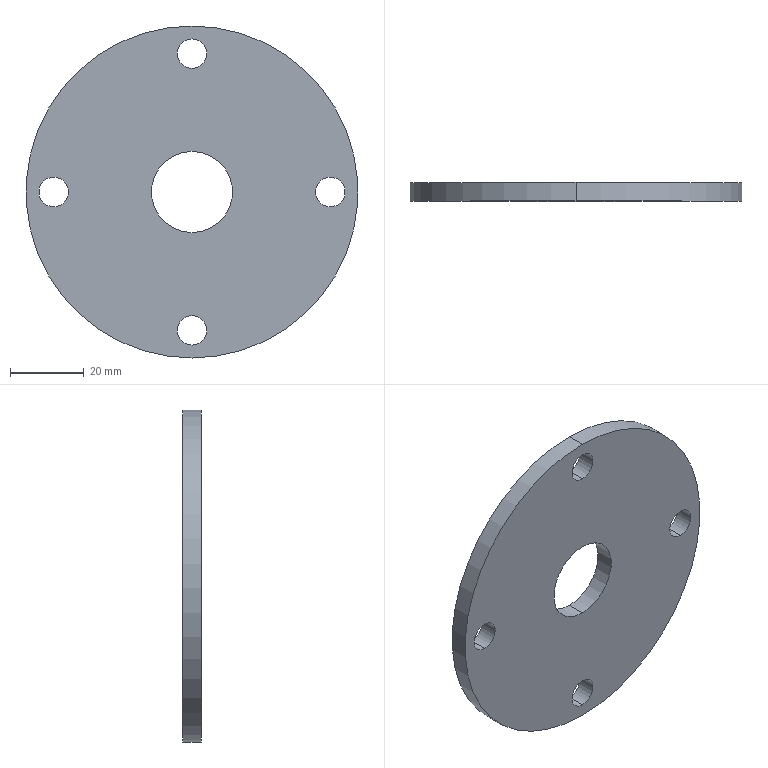Part | STEP file | Guide wheel mechanism revised.sldasm-Part-427 | 1 solid | 34 faces | box 90 x 5 x 90 mm | volume 28260 mm3 | plane 22 | cylinder 12 | commonest cylinder face diameters 8 x8 22 x2 90 x2
STEP:
#1=CARTESIAN_POINT('',(37.5,5.,-4.));
#2=VERTEX_POINT('',#1);
#3=CARTESIAN_POINT('',(37.5,5.,4.));
#4=VERTEX_POINT('',#3);
#5=CARTESIAN_POINT('',(37.5,5.,0.));
#6=DIRECTION('',(0.,1.,0.));
#7=DIRECTION('',(0.,0.,1.));
#8=AXIS2_PLACEMENT_3D('',#5,#6,#7);
#9=CIRCLE('',#8,4.);
#10=EDGE_CURVE('',#2,#4,#9,.T.);
#11=ORIENTED_EDGE('',*,*,#10,.T.);
#12=CARTESIAN_POINT('',(37.5,0.,4.));
#13=VERTEX_POINT('',#12);
#14=CARTESIAN_POINT('',(37.5,5.,4.));
#15=DIRECTION('',(0.,-1.,0.));
#16=VECTOR('',#15,1000.);
#17=LINE('',#14,#16);
#18=EDGE_CURVE('',#4,#13,#17,.T.);
#19=ORIENTED_EDGE('',*,*,#18,.T.);
#20=CARTESIAN_POINT('',(37.5,0.,-4.));
#21=VERTEX_POINT('',#20);
#22=CARTESIAN_POINT('',(37.5,0.,0.));
#23=DIRECTION('',(0.,1.,0.));
#24=DIRECTION('',(0.,0.,1.));
#25=AXIS2_PLACEMENT_3D('',#22,#23,#24);
#26=CIRCLE('',#25,4.);
#27=EDGE_CURVE('',#21,#13,#26,.T.);
#28=ORIENTED_EDGE('',*,*,#27,.F.);
#29=CARTESIAN_POINT('',(37.5,5.,-4.));
#30=DIRECTION('',(0.,-1.,0.));
#31=VECTOR('',#30,1000.);
#32=LINE('',#29,#31);
#33=EDGE_CURVE('',#2,#21,#32,.T.);
#34=ORIENTED_EDGE('',*,*,#33,.F.);
#35=EDGE_LOOP('',(#11,#19,#28,#34));
#36=FACE_OUTER_BOUND('',#35,.T.);
#37=CARTESIAN_POINT('',(37.5,5.,0.));
#38=DIRECTION('',(0.,-1.,0.));
#39=DIRECTION('',(0.,0.,-1.));
#40=AXIS2_PLACEMENT_3D('',#37,#38,#39);
#41=CYLINDRICAL_SURFACE('',#40,4.);
#42=ADVANCED_FACE('',(#36),#41,.F.);
#43=CARTESIAN_POINT('',(0.,5.,33.5));
#44=VERTEX_POINT('',#43);
#45=CARTESIAN_POINT('',(0.,5.,41.5));
#46=VERTEX_POINT('',#45);
#47=CARTESIAN_POINT('',(0.,5.,37.5));
#48=DIRECTION('',(0.,1.,0.));
#49=DIRECTION('',(0.,0.,1.));
#50=AXIS2_PLACEMENT_3D('',#47,#48,#49);
#51=CIRCLE('',#50,4.);
#52=EDGE_CURVE('',#44,#46,#51,.T.);
#53=ORIENTED_EDGE('',*,*,#52,.T.);
#54=CARTESIAN_POINT('',(0.,0.,41.5));
#55=VERTEX_POINT('',#54);
#56=CARTESIAN_POINT('',(0.,5.,41.5));
#57=DIRECTION('',(0.,-1.,0.));
#58=VECTOR('',#57,1000.);
#59=LINE('',#56,#58);
#60=EDGE_CURVE('',#46,#55,#59,.T.);
#61=ORIENTED_EDGE('',*,*,#60,.T.);
#62=CARTESIAN_POINT('',(0.,0.,33.5));
#63=VERTEX_POINT('',#62);
#64=CARTESIAN_POINT('',(0.,0.,37.5));
#65=DIRECTION('',(0.,1.,0.));
#66=DIRECTION('',(0.,0.,1.));
#67=AXIS2_PLACEMENT_3D('',#64,#65,#66);
#68=CIRCLE('',#67,4.);
#69=EDGE_CURVE('',#63,#55,#68,.T.);
#70=ORIENTED_EDGE('',*,*,#69,.F.);
#71=CARTESIAN_POINT('',(0.,5.,33.5));
#72=DIRECTION('',(0.,-1.,0.));
#73=VECTOR('',#72,1000.);
#74=LINE('',#71,#73);
#75=EDGE_CURVE('',#44,#63,#74,.T.);
#76=ORIENTED_EDGE('',*,*,#75,.F.);
#77=EDGE_LOOP('',(#53,#61,#70,#76));
#78=FACE_OUTER_BOUND('',#77,.T.);
#79=CARTESIAN_POINT('',(0.,5.,37.5));
#80=DIRECTION('',(0.,-1.,0.));
#81=DIRECTION('',(0.,0.,-1.));
#82=AXIS2_PLACEMENT_3D('',#79,#80,#81);
#83=CYLINDRICAL_SURFACE('',#82,4.);
#84=ADVANCED_FACE('',(#78),#83,.F.);
#85=CARTESIAN_POINT('',(-37.5,5.,-4.));
#86=VERTEX_POINT('',#85);
#87=CARTESIAN_POINT('',(-37.5,5.,4.));
#88=VERTEX_POINT('',#87);
#89=CARTESIAN_POINT('',(-37.5,5.,0.));
#90=DIRECTION('',(0.,1.,0.));
#91=DIRECTION('',(0.,0.,1.));
#92=AXIS2_PLACEMENT_3D('',#89,#90,#91);
#93=CIRCLE('',#92,4.);
#94=EDGE_CURVE('',#86,#88,#93,.T.);
#95=ORIENTED_EDGE('',*,*,#94,.T.);
#96=CARTESIAN_POINT('',(-37.5,0.,4.));
#97=VERTEX_POINT('',#96);
#98=CARTESIAN_POINT('',(-37.5,5.,4.));
#99=DIRECTION('',(0.,-1.,0.));
#100=VECTOR('',#99,1000.);
#101=LINE('',#98,#100);
#102=EDGE_CURVE('',#88,#97,#101,.T.);
#103=ORIENTED_EDGE('',*,*,#102,.T.);
#104=CARTESIAN_POINT('',(-37.5,0.,-4.));
#105=VERTEX_POINT('',#104);
#106=CARTESIAN_POINT('',(-37.5,0.,0.));
#107=DIRECTION('',(0.,1.,0.));
#108=DIRECTION('',(0.,0.,1.));
#109=AXIS2_PLACEMENT_3D('',#106,#107,#108);
#110=CIRCLE('',#109,4.);
#111=EDGE_CURVE('',#105,#97,#110,.T.);
#112=ORIENTED_EDGE('',*,*,#111,.F.);
#113=CARTESIAN_POINT('',(-37.5,5.,-4.));
#114=DIRECTION('',(0.,-1.,0.));
#115=VECTOR('',#114,1000.);
#116=LINE('',#113,#115);
#117=EDGE_CURVE('',#86,#105,#116,.T.);
#118=ORIENTED_EDGE('',*,*,#117,.F.);
#119=EDGE_LOOP('',(#95,#103,#112,#118));
#120=FACE_OUTER_BOUND('',#119,.T.);
#121=CARTESIAN_POINT('',(-37.5,5.,0.));
#122=DIRECTION('',(0.,-1.,0.));
#123=DIRECTION('',(0.,0.,-1.));
#124=AXIS2_PLACEMENT_3D('',#121,#122,#123);
#125=CYLINDRICAL_SURFACE('',#124,4.);
#126=ADVANCED_FACE('',(#120),#125,.F.);
#127=CARTESIAN_POINT('',(0.,5.,-41.5));
#128=VERTEX_POINT('',#127);
#129=CARTESIAN_POINT('',(0.,5.,-33.5));
#130=VERTEX_POINT('',#129);
#131=CARTESIAN_POINT('',(0.,5.,-37.5));
#132=DIRECTION('',(0.,1.,0.));
#133=DIRECTION('',(0.,0.,1.));
#134=AXIS2_PLACEMENT_3D('',#131,#132,#133);
#135=CIRCLE('',#134,4.);
#136=EDGE_CURVE('',#128,#130,#135,.T.);
#137=ORIENTED_EDGE('',*,*,#136,.T.);
#138=CARTESIAN_POINT('',(0.,0.,-33.5));
#139=VERTEX_POINT('',#138);
#140=CARTESIAN_POINT('',(0.,5.,-33.5));
#141=DIRECTION('',(0.,-1.,0.));
#142=VECTOR('',#141,1000.);
#143=LINE('',#140,#142);
#144=EDGE_CURVE('',#130,#139,#143,.T.);
#145=ORIENTED_EDGE('',*,*,#144,.T.);
#146=CARTESIAN_POINT('',(0.,0.,-41.5));
#147=VERTEX_POINT('',#146);
#148=CARTESIAN_POINT('',(0.,0.,-37.5));
#149=DIRECTION('',(0.,1.,0.));
#150=DIRECTION('',(0.,0.,1.));
#151=AXIS2_PLACEMENT_3D('',#148,#149,#150);
#152=CIRCLE('',#151,4.);
#153=EDGE_CURVE('',#147,#139,#152,.T.);
#154=ORIENTED_EDGE('',*,*,#153,.F.);
#155=CARTESIAN_POINT('',(0.,5.,-41.5));
#156=DIRECTION('',(0.,-1.,0.));
#157=VECTOR('',#156,1000.);
#158=LINE('',#155,#157);
#159=EDGE_CURVE('',#128,#147,#158,.T.);
#160=ORIENTED_EDGE('',*,*,#159,.F.);
#161=EDGE_LOOP('',(#137,#145,#154,#160));
#162=FACE_OUTER_BOUND('',#161,.T.);
#163=CARTESIAN_POINT('',(0.,5.,-37.5));
#164=DIRECTION('',(0.,-1.,0.));
#165=DIRECTION('',(0.,0.,-1.));
#166=AXIS2_PLACEMENT_3D('',#163,#164,#165);
#167=CYLINDRICAL_SURFACE('',#166,4.);
#168=ADVANCED_FACE('',(#162),#167,.F.);
#169=CARTESIAN_POINT('',(0.,5.,-11.));
#170=VERTEX_POINT('',#169);
#171=CARTESIAN_POINT('',(0.,5.,11.));
#172=VERTEX_POINT('',#171);
#173=CARTESIAN_POINT('',(0.,5.,0.));
#174=DIRECTION('',(0.,1.,0.));
#175=DIRECTION('',(0.,0.,1.));
#176=AXIS2_PLACEMENT_3D('',#173,#174,#175);
#177=CIRCLE('',#176,11.);
#178=EDGE_CURVE('',#170,#172,#177,.T.);
#179=ORIENTED_EDGE('',*,*,#178,.T.);
#180=CARTESIAN_POINT('',(0.,0.,11.));
#181=VERTEX_POINT('',#180);
#182=CARTESIAN_POINT('',(0.,5.,11.));
#183=DIRECTION('',(0.,-1.,0.));
#184=VECTOR('',#183,1000.);
#185=LINE('',#182,#184);
#186=EDGE_CURVE('',#172,#181,#185,.T.);
#187=ORIENTED_EDGE('',*,*,#186,.T.);
#188=CARTESIAN_POINT('',(0.,0.,-11.));
#189=VERTEX_POINT('',#188);
#190=CARTESIAN_POINT('',(0.,0.,0.));
#191=DIRECTION('',(0.,1.,0.));
#192=DIRECTION('',(0.,0.,1.));
#193=AXIS2_PLACEMENT_3D('',#190,#191,#192);
#194=CIRCLE('',#193,11.);
#195=EDGE_CURVE('',#189,#181,#194,.T.);
#196=ORIENTED_EDGE('',*,*,#195,.F.);
#197=CARTESIAN_POINT('',(0.,5.,-11.));
#198=DIRECTION('',(0.,-1.,0.));
#199=VECTOR('',#198,1000.);
#200=LINE('',#197,#199);
#201=EDGE_CURVE('',#170,#189,#200,.T.);
#202=ORIENTED_EDGE('',*,*,#201,.F.);
#203=EDGE_LOOP('',(#179,#187,#196,#202));
#204=FACE_OUTER_BOUND('',#203,.T.);
#205=CARTESIAN_POINT('',(0.,5.,0.));
#206=DIRECTION('',(0.,-1.,0.));
#207=DIRECTION('',(0.,0.,-1.));
#208=AXIS2_PLACEMENT_3D('',#205,#206,#207);
#209=CYLINDRICAL_SURFACE('',#208,11.);
#210=ADVANCED_FACE('',(#204),#209,.F.);
#211=CARTESIAN_POINT('',(0.,5.,45.));
#212=VERTEX_POINT('',#211);
#213=CARTESIAN_POINT('',(0.,5.,-45.));
#214=VERTEX_POINT('',#213);
#215=CARTESIAN_POINT('',(0.,5.,0.));
#216=DIRECTION('',(0.,1.,0.));
#217=DIRECTION('',(0.,0.,1.));
#218=AXIS2_PLACEMENT_3D('',#215,#216,#217);
#219=CIRCLE('',#218,45.);
#220=EDGE_CURVE('',#212,#214,#219,.T.);
#221=ORIENTED_EDGE('',*,*,#220,.F.);
#222=CARTESIAN_POINT('',(0.,0.,45.));
#223=VERTEX_POINT('',#222);
#224=CARTESIAN_POINT('',(0.,5.,45.));
#225=DIRECTION('',(0.,-1.,0.));
#226=VECTOR('',#225,1000.);
#227=LINE('',#224,#226);
#228=EDGE_CURVE('',#212,#223,#227,.T.);
#229=ORIENTED_EDGE('',*,*,#228,.T.);
#230=CARTESIAN_POINT('',(0.,0.,-45.));
#231=VERTEX_POINT('',#230);
#232=CARTESIAN_POINT('',(0.,0.,0.));
#233=DIRECTION('',(0.,1.,0.));
#234=DIRECTION('',(0.,0.,1.));
#235=AXIS2_PLACEMENT_3D('',#232,#233,#234);
#236=CIRCLE('',#235,45.);
#237=EDGE_CURVE('',#223,#231,#236,.T.);
#238=ORIENTED_EDGE('',*,*,#237,.T.);
#239=CARTESIAN_POINT('',(0.,5.,-45.));
#240=DIRECTION('',(0.,-1.,0.));
#241=VECTOR('',#240,1000.);
#242=LINE('',#239,#241);
#243=EDGE_CURVE('',#214,#231,#242,.T.);
#244=ORIENTED_EDGE('',*,*,#243,.F.);
#245=EDGE_LOOP('',(#221,#229,#238,#244));
#246=FACE_OUTER_BOUND('',#245,.T.);
#247=CARTESIAN_POINT('',(0.,5.,0.));
#248=DIRECTION('',(0.,-1.,0.));
#249=DIRECTION('',(0.,0.,-1.));
#250=AXIS2_PLACEMENT_3D('',#247,#248,#249);
#251=CYLINDRICAL_SURFACE('',#250,45.);
#252=ADVANCED_FACE('',(#246),#251,.T.);
#253=CARTESIAN_POINT('',(-22.309,5.,26.198));
#254=VERTEX_POINT('',#253);
#255=CARTESIAN_POINT('',(-17.147,5.,21.036));
#256=VERTEX_POINT('',#255);
#257=CARTESIAN_POINT('',(1.945,5.,1.945));
#258=DIRECTION('',(0.7071,0.,-0.7071));
#259=VECTOR('',#258,1000.);
#260=LINE('',#257,#259);
#261=EDGE_CURVE('',#254,#256,#260,.T.);
#262=ORIENTED_EDGE('',*,*,#261,.F.);
#263=CARTESIAN_POINT('',(-26.198,5.,22.309));
#264=VERTEX_POINT('',#263);
#265=CARTESIAN_POINT('',(-24.254,5.,24.254));
#266=DIRECTION('',(0.7071,0.,0.7071));
#267=VECTOR('',#266,1000.);
#268=LINE('',#265,#267);
#269=EDGE_CURVE('',#264,#254,#268,.T.);
#270=ORIENTED_EDGE('',*,*,#269,.F.);
#271=CARTESIAN_POINT('',(-21.036,5.,17.147));
#272=VERTEX_POINT('',#271);
#273=CARTESIAN_POINT('',(-1.945,5.,-1.945));
#274=DIRECTION('',(0.7071,0.,-0.7071));
#275=VECTOR('',#274,1000.);
#276=LINE('',#273,#275);
#277=EDGE_CURVE('',#264,#272,#276,.T.);
#278=ORIENTED_EDGE('',*,*,#277,.T.);
#279=CARTESIAN_POINT('',(-19.092,5.,19.092));
#280=DIRECTION('',(0.7071,0.,0.7071));
#281=VECTOR('',#280,1000.);
#282=LINE('',#279,#281);
#283=EDGE_CURVE('',#272,#256,#282,.T.);
#284=ORIENTED_EDGE('',*,*,#283,.T.);
#285=EDGE_LOOP('',(#262,#270,#278,#284));
#286=FACE_BOUND('',#285,.T.);
#287=CARTESIAN_POINT('',(26.198,5.,22.309));
#288=VERTEX_POINT('',#287);
#289=CARTESIAN_POINT('',(21.036,5.,17.147));
#290=VERTEX_POINT('',#289);
#291=CARTESIAN_POINT('',(1.945,5.,-1.945));
#292=DIRECTION('',(-0.7071,0.,-0.7071));
#293=VECTOR('',#292,1000.);
#294=LINE('',#291,#293);
#295=EDGE_CURVE('',#288,#290,#294,.T.);
#296=ORIENTED_EDGE('',*,*,#295,.F.);
#297=CARTESIAN_POINT('',(22.309,5.,26.198));
#298=VERTEX_POINT('',#297);
#299=CARTESIAN_POINT('',(24.254,5.,24.254));
#300=DIRECTION('',(0.7071,0.,-0.7071));
#301=VECTOR('',#300,1000.);
#302=LINE('',#299,#301);
#303=EDGE_CURVE('',#298,#288,#302,.T.);
#304=ORIENTED_EDGE('',*,*,#303,.F.);
#305=CARTESIAN_POINT('',(17.147,5.,21.036));
#306=VERTEX_POINT('',#305);
#307=CARTESIAN_POINT('',(-1.945,5.,1.945));
#308=DIRECTION('',(-0.7071,0.,-0.7071));
#309=VECTOR('',#308,1000.);
#310=LINE('',#307,#309);
#311=EDGE_CURVE('',#298,#306,#310,.T.);
#312=ORIENTED_EDGE('',*,*,#311,.T.);
#313=CARTESIAN_POINT('',(19.092,5.,19.092));
#314=DIRECTION('',(0.7071,0.,-0.7071));
#315=VECTOR('',#314,1000.);
#316=LINE('',#313,#315);
#317=EDGE_CURVE('',#306,#290,#316,.T.);
#318=ORIENTED_EDGE('',*,*,#317,.T.);
#319=EDGE_LOOP('',(#296,#304,#312,#318));
#320=FACE_BOUND('',#319,.T.);
#321=CARTESIAN_POINT('',(22.309,5.,-26.198));
#322=VERTEX_POINT('',#321);
#323=CARTESIAN_POINT('',(17.147,5.,-21.036));
#324=VERTEX_POINT('',#323);
#325=CARTESIAN_POINT('',(-1.945,5.,-1.945));
#326=DIRECTION('',(-0.7071,0.,0.7071));
#327=VECTOR('',#326,1000.);
#328=LINE('',#325,#327);
#329=EDGE_CURVE('',#322,#324,#328,.T.);
#330=ORIENTED_EDGE('',*,*,#329,.F.);
#331=CARTESIAN_POINT('',(26.198,5.,-22.309));
#332=VERTEX_POINT('',#331);
#333=CARTESIAN_POINT('',(24.254,5.,-24.254));
#334=DIRECTION('',(-0.7071,0.,-0.7071));
#335=VECTOR('',#334,1000.);
#336=LINE('',#333,#335);
#337=EDGE_CURVE('',#332,#322,#336,.T.);
#338=ORIENTED_EDGE('',*,*,#337,.F.);
#339=CARTESIAN_POINT('',(21.036,5.,-17.147));
#340=VERTEX_POINT('',#339);
#341=CARTESIAN_POINT('',(1.945,5.,1.945));
#342=DIRECTION('',(-0.7071,0.,0.7071));
#343=VECTOR('',#342,1000.);
#344=LINE('',#341,#343);
#345=EDGE_CURVE('',#332,#340,#344,.T.);
#346=ORIENTED_EDGE('',*,*,#345,.T.);
#347=CARTESIAN_POINT('',(19.092,5.,-19.092));
#348=DIRECTION('',(-0.7071,0.,-0.7071));
#349=VECTOR('',#348,1000.);
#350=LINE('',#347,#349);
#351=EDGE_CURVE('',#340,#324,#350,.T.);
#352=ORIENTED_EDGE('',*,*,#351,.T.);
#353=EDGE_LOOP('',(#330,#338,#346,#352));
#354=FACE_BOUND('',#353,.T.);
#355=CARTESIAN_POINT('',(-26.198,5.,-22.309));
#356=VERTEX_POINT('',#355);
#357=CARTESIAN_POINT('',(-21.036,5.,-17.147));
#358=VERTEX_POINT('',#357);
#359=CARTESIAN_POINT('',(-1.945,5.,1.945));
#360=DIRECTION('',(0.7071,0.,0.7071));
#361=VECTOR('',#360,1000.);
#362=LINE('',#359,#361);
#363=EDGE_CURVE('',#356,#358,#362,.T.);
#364=ORIENTED_EDGE('',*,*,#363,.F.);
#365=CARTESIAN_POINT('',(-22.309,5.,-26.198));
#366=VERTEX_POINT('',#365);
#367=CARTESIAN_POINT('',(-24.254,5.,-24.254));
#368=DIRECTION('',(-0.7071,0.,0.7071));
#369=VECTOR('',#368,1000.);
#370=LINE('',#367,#369);
#371=EDGE_CURVE('',#366,#356,#370,.T.);
#372=ORIENTED_EDGE('',*,*,#371,.F.);
#373=CARTESIAN_POINT('',(-17.147,5.,-21.036));
#374=VERTEX_POINT('',#373);
#375=CARTESIAN_POINT('',(1.945,5.,-1.945));
#376=DIRECTION('',(0.7071,0.,0.7071));
#377=VECTOR('',#376,1000.);
#378=LINE('',#375,#377);
#379=EDGE_CURVE('',#366,#374,#378,.T.);
#380=ORIENTED_EDGE('',*,*,#379,.T.);
#381=CARTESIAN_POINT('',(-19.092,5.,-19.092));
#382=DIRECTION('',(-0.7071,0.,0.7071));
#383=VECTOR('',#382,1000.);
#384=LINE('',#381,#383);
#385=EDGE_CURVE('',#374,#358,#384,.T.);
#386=ORIENTED_EDGE('',*,*,#385,.T.);
#387=EDGE_LOOP('',(#364,#372,#380,#386));
#388=FACE_BOUND('',#387,.T.);
#389=ORIENTED_EDGE('',*,*,#52,.F.);
#390=CARTESIAN_POINT('',(0.,5.,37.5));
#391=DIRECTION('',(0.,1.,0.));
#392=DIRECTION('',(0.,0.,1.));
#393=AXIS2_PLACEMENT_3D('',#390,#391,#392);
#394=CIRCLE('',#393,4.);
#395=EDGE_CURVE('',#46,#44,#394,.T.);
#396=ORIENTED_EDGE('',*,*,#395,.F.);
#397=EDGE_LOOP('',(#389,#396));
#398=FACE_BOUND('',#397,.T.);
#399=ORIENTED_EDGE('',*,*,#136,.F.);
#400=CARTESIAN_POINT('',(0.,5.,-37.5));
#401=DIRECTION('',(0.,1.,0.));
#402=DIRECTION('',(0.,0.,1.));
#403=AXIS2_PLACEMENT_3D('',#400,#401,#402);
#404=CIRCLE('',#403,4.);
#405=EDGE_CURVE('',#130,#128,#404,.T.);
#406=ORIENTED_EDGE('',*,*,#405,.F.);
#407=EDGE_LOOP('',(#399,#406));
#408=FACE_BOUND('',#407,.T.);
#409=CARTESIAN_POINT('',(0.,5.,0.));
#410=DIRECTION('',(0.,1.,0.));
#411=DIRECTION('',(0.,0.,1.));
#412=AXIS2_PLACEMENT_3D('',#409,#410,#411);
#413=CIRCLE('',#412,45.);
#414=EDGE_CURVE('',#214,#212,#413,.T.);
#415=ORIENTED_EDGE('',*,*,#414,.T.);
#416=ORIENTED_EDGE('',*,*,#220,.T.);
#417=EDGE_LOOP('',(#415,#416));
#418=FACE_OUTER_BOUND('',#417,.T.);
#419=ORIENTED_EDGE('',*,*,#178,.F.);
#420=CARTESIAN_POINT('',(0.,5.,0.));
#421=DIRECTION('',(0.,1.,0.));
#422=DIRECTION('',(0.,0.,1.));
#423=AXIS2_PLACEMENT_3D('',#420,#421,#422);
#424=CIRCLE('',#423,11.);
#425=EDGE_CURVE('',#172,#170,#424,.T.);
#426=ORIENTED_EDGE('',*,*,#425,.F.);
#427=EDGE_LOOP('',(#419,#426));
#428=FACE_BOUND('',#427,.T.);
#429=ORIENTED_EDGE('',*,*,#94,.F.);
#430=CARTESIAN_POINT('',(-37.5,5.,0.));
#431=DIRECTION('',(0.,1.,0.));
#432=DIRECTION('',(0.,0.,1.));
#433=AXIS2_PLACEMENT_3D('',#430,#431,#432);
#434=CIRCLE('',#433,4.);
#435=EDGE_CURVE('',#88,#86,#434,.T.);
#436=ORIENTED_EDGE('',*,*,#435,.F.);
#437=EDGE_LOOP('',(#429,#436));
#438=FACE_BOUND('',#437,.T.);
#439=ORIENTED_EDGE('',*,*,#10,.F.);
#440=CARTESIAN_POINT('',(37.5,5.,0.));
#441=DIRECTION('',(0.,1.,0.));
#442=DIRECTION('',(0.,0.,1.));
#443=AXIS2_PLACEMENT_3D('',#440,#441,#442);
#444=CIRCLE('',#443,4.);
#445=EDGE_CURVE('',#4,#2,#444,.T.);
#446=ORIENTED_EDGE('',*,*,#445,.F.);
#447=EDGE_LOOP('',(#439,#446));
#448=FACE_BOUND('',#447,.T.);
#449=CARTESIAN_POINT('',(0.,5.,0.));
#450=DIRECTION('',(0.,1.,0.));
#451=DIRECTION('',(0.,0.,1.));
#452=AXIS2_PLACEMENT_3D('',#449,#450,#451);
#453=PLANE('',#452);
#454=ADVANCED_FACE('',(#286,#320,#354,#388,#398,#408,#418,#428,#438,#448),#453,.T.);
#455=ORIENTED_EDGE('',*,*,#69,.T.);
#456=CARTESIAN_POINT('',(0.,0.,37.5));
#457=DIRECTION('',(0.,1.,0.));
#458=DIRECTION('',(0.,0.,1.));
#459=AXIS2_PLACEMENT_3D('',#456,#457,#458);
#460=CIRCLE('',#459,4.);
#461=EDGE_CURVE('',#55,#63,#460,.T.);
#462=ORIENTED_EDGE('',*,*,#461,.T.);
#463=EDGE_LOOP('',(#455,#462));
#464=FACE_BOUND('',#463,.T.);
#465=ORIENTED_EDGE('',*,*,#153,.T.);
#466=CARTESIAN_POINT('',(0.,0.,-37.5));
#467=DIRECTION('',(0.,1.,0.));
#468=DIRECTION('',(0.,0.,1.));
#469=AXIS2_PLACEMENT_3D('',#466,#467,#468);
#470=CIRCLE('',#469,4.);
#471=EDGE_CURVE('',#139,#147,#470,.T.);
#472=ORIENTED_EDGE('',*,*,#471,.T.);
#473=EDGE_LOOP('',(#465,#472));
#474=FACE_BOUND('',#473,.T.);
#475=CARTESIAN_POINT('',(0.,0.,0.));
#476=DIRECTION('',(0.,1.,0.));
#477=DIRECTION('',(0.,0.,1.));
#478=AXIS2_PLACEMENT_3D('',#475,#476,#477);
#479=CIRCLE('',#478,45.);
#480=EDGE_CURVE('',#231,#223,#479,.T.);
#481=ORIENTED_EDGE('',*,*,#480,.F.);
#482=ORIENTED_EDGE('',*,*,#237,.F.);
#483=EDGE_LOOP('',(#481,#482));
#484=FACE_OUTER_BOUND('',#483,.T.);
#485=ORIENTED_EDGE('',*,*,#195,.T.);
#486=CARTESIAN_POINT('',(0.,0.,0.));
#487=DIRECTION('',(0.,1.,0.));
#488=DIRECTION('',(0.,0.,1.));
#489=AXIS2_PLACEMENT_3D('',#486,#487,#488);
#490=CIRCLE('',#489,11.);
#491=EDGE_CURVE('',#181,#189,#490,.T.);
#492=ORIENTED_EDGE('',*,*,#491,.T.);
#493=EDGE_LOOP('',(#485,#492));
#494=FACE_BOUND('',#493,.T.);
#495=ORIENTED_EDGE('',*,*,#111,.T.);
#496=CARTESIAN_POINT('',(-37.5,0.,0.));
#497=DIRECTION('',(0.,1.,0.));
#498=DIRECTION('',(0.,0.,1.));
#499=AXIS2_PLACEMENT_3D('',#496,#497,#498);
#500=CIRCLE('',#499,4.);
#501=EDGE_CURVE('',#97,#105,#500,.T.);
#502=ORIENTED_EDGE('',*,*,#501,.T.);
#503=EDGE_LOOP('',(#495,#502));
#504=FACE_BOUND('',#503,.T.);
#505=ORIENTED_EDGE('',*,*,#27,.T.);
#506=CARTESIAN_POINT('',(37.5,0.,0.));
#507=DIRECTION('',(0.,1.,0.));
#508=DIRECTION('',(0.,0.,1.));
#509=AXIS2_PLACEMENT_3D('',#506,#507,#508);
#510=CIRCLE('',#509,4.);
#511=EDGE_CURVE('',#13,#21,#510,.T.);
#512=ORIENTED_EDGE('',*,*,#511,.T.);
#513=EDGE_LOOP('',(#505,#512));
#514=FACE_BOUND('',#513,.T.);
#515=CARTESIAN_POINT('',(0.,0.,0.));
#516=DIRECTION('',(0.,1.,0.));
#517=DIRECTION('',(0.,0.,1.));
#518=AXIS2_PLACEMENT_3D('',#515,#516,#517);
#519=PLANE('',#518);
#520=ADVANCED_FACE('',(#464,#474,#484,#494,#504,#514),#519,.F.);
#521=ORIENTED_EDGE('',*,*,#228,.F.);
#522=ORIENTED_EDGE('',*,*,#414,.F.);
#523=ORIENTED_EDGE('',*,*,#243,.T.);
#524=ORIENTED_EDGE('',*,*,#480,.T.);
#525=EDGE_LOOP('',(#521,#522,#523,#524));
#526=FACE_OUTER_BOUND('',#525,.T.);
#527=CARTESIAN_POINT('',(0.,5.,0.));
#528=DIRECTION('',(0.,-1.,0.));
#529=DIRECTION('',(0.,0.,-1.));
#530=AXIS2_PLACEMENT_3D('',#527,#528,#529);
#531=CYLINDRICAL_SURFACE('',#530,45.);
#532=ADVANCED_FACE('',(#526),#531,.T.);
#533=ORIENTED_EDGE('',*,*,#186,.F.);
#534=ORIENTED_EDGE('',*,*,#425,.T.);
#535=ORIENTED_EDGE('',*,*,#201,.T.);
#536=ORIENTED_EDGE('',*,*,#491,.F.);
#537=EDGE_LOOP('',(#533,#534,#535,#536));
#538=FACE_OUTER_BOUND('',#537,.T.);
#539=CARTESIAN_POINT('',(0.,5.,0.));
#540=DIRECTION('',(0.,-1.,0.));
#541=DIRECTION('',(0.,0.,-1.));
#542=AXIS2_PLACEMENT_3D('',#539,#540,#541);
#543=CYLINDRICAL_SURFACE('',#542,11.);
#544=ADVANCED_FACE('',(#538),#543,.F.);
#545=ORIENTED_EDGE('',*,*,#144,.F.);
#546=ORIENTED_EDGE('',*,*,#405,.T.);
#547=ORIENTED_EDGE('',*,*,#159,.T.);
#548=ORIENTED_EDGE('',*,*,#471,.F.);
#549=EDGE_LOOP('',(#545,#546,#547,#548));
#550=FACE_OUTER_BOUND('',#549,.T.);
#551=CARTESIAN_POINT('',(0.,5.,-37.5));
#552=DIRECTION('',(0.,-1.,0.));
#553=DIRECTION('',(0.,0.,-1.));
#554=AXIS2_PLACEMENT_3D('',#551,#552,#553);
#555=CYLINDRICAL_SURFACE('',#554,4.);
#556=ADVANCED_FACE('',(#550),#555,.F.);
#557=ORIENTED_EDGE('',*,*,#102,.F.);
#558=ORIENTED_EDGE('',*,*,#435,.T.);
#559=ORIENTED_EDGE('',*,*,#117,.T.);
#560=ORIENTED_EDGE('',*,*,#501,.F.);
#561=EDGE_LOOP('',(#557,#558,#559,#560));
#562=FACE_OUTER_BOUND('',#561,.T.);
#563=CARTESIAN_POINT('',(-37.5,5.,0.));
#564=DIRECTION('',(0.,-1.,0.));
#565=DIRECTION('',(0.,0.,-1.));
#566=AXIS2_PLACEMENT_3D('',#563,#564,#565);
#567=CYLINDRICAL_SURFACE('',#566,4.);
#568=ADVANCED_FACE('',(#562),#567,.F.);
#569=ORIENTED_EDGE('',*,*,#60,.F.);
#570=ORIENTED_EDGE('',*,*,#395,.T.);
#571=ORIENTED_EDGE('',*,*,#75,.T.);
#572=ORIENTED_EDGE('',*,*,#461,.F.);
#573=EDGE_LOOP('',(#569,#570,#571,#572));
#574=FACE_OUTER_BOUND('',#573,.T.);
#575=CARTESIAN_POINT('',(0.,5.,37.5));
#576=DIRECTION('',(0.,-1.,0.));
#577=DIRECTION('',(0.,0.,-1.));
#578=AXIS2_PLACEMENT_3D('',#575,#576,#577);
#579=CYLINDRICAL_SURFACE('',#578,4.);
#580=ADVANCED_FACE('',(#574),#579,.F.);
#581=ORIENTED_EDGE('',*,*,#18,.F.);
#582=ORIENTED_EDGE('',*,*,#445,.T.);
#583=ORIENTED_EDGE('',*,*,#33,.T.);
#584=ORIENTED_EDGE('',*,*,#511,.F.);
#585=EDGE_LOOP('',(#581,#582,#583,#584));
#586=FACE_OUTER_BOUND('',#585,.T.);
#587=CARTESIAN_POINT('',(37.5,5.,0.));
#588=DIRECTION('',(0.,-1.,0.));
#589=DIRECTION('',(0.,0.,-1.));
#590=AXIS2_PLACEMENT_3D('',#587,#588,#589);
#591=CYLINDRICAL_SURFACE('',#590,4.);
#592=ADVANCED_FACE('',(#586),#591,.F.);
#593=ORIENTED_EDGE('',*,*,#363,.T.);
#594=CARTESIAN_POINT('',(-21.036,1.,-17.147));
#595=VERTEX_POINT('',#594);
#596=CARTESIAN_POINT('',(-21.036,1.,-17.147));
#597=DIRECTION('',(0.,1.,0.));
#598=VECTOR('',#597,1000.);
#599=LINE('',#596,#598);
#600=EDGE_CURVE('',#595,#358,#599,.T.);
#601=ORIENTED_EDGE('',*,*,#600,.F.);
#602=CARTESIAN_POINT('',(-26.198,1.,-22.309));
#603=VERTEX_POINT('',#602);
#604=CARTESIAN_POINT('',(-1.945,1.,1.945));
#605=DIRECTION('',(0.7071,0.,0.7071));
#606=VECTOR('',#605,1000.);
#607=LINE('',#604,#606);
#608=EDGE_CURVE('',#603,#595,#607,.T.);
#609=ORIENTED_EDGE('',*,*,#608,.F.);
#610=CARTESIAN_POINT('',(-26.198,1.,-22.309));
#611=DIRECTION('',(0.,1.,0.));
#612=VECTOR('',#611,1000.);
#613=LINE('',#610,#612);
#614=EDGE_CURVE('',#603,#356,#613,.T.);
#615=ORIENTED_EDGE('',*,*,#614,.T.);
#616=EDGE_LOOP('',(#593,#601,#609,#615));
#617=FACE_OUTER_BOUND('',#616,.T.);
#618=CARTESIAN_POINT('',(-1.945,1.,1.945));
#619=DIRECTION('',(-0.7071,0.,0.7071));
#620=DIRECTION('',(0.7071,0.,0.7071));
#621=AXIS2_PLACEMENT_3D('',#618,#619,#620);
#622=PLANE('',#621);
#623=ADVANCED_FACE('',(#617),#622,.F.);
#624=ORIENTED_EDGE('',*,*,#371,.T.);
#625=ORIENTED_EDGE('',*,*,#614,.F.);
#626=CARTESIAN_POINT('',(-22.309,1.,-26.198));
#627=VERTEX_POINT('',#626);
#628=CARTESIAN_POINT('',(-24.254,1.,-24.254));
#629=DIRECTION('',(-0.7071,0.,0.7071));
#630=VECTOR('',#629,1000.);
#631=LINE('',#628,#630);
#632=EDGE_CURVE('',#627,#603,#631,.T.);
#633=ORIENTED_EDGE('',*,*,#632,.F.);
#634=CARTESIAN_POINT('',(-22.309,1.,-26.198));
#635=DIRECTION('',(0.,1.,0.));
#636=VECTOR('',#635,1000.);
#637=LINE('',#634,#636);
#638=EDGE_CURVE('',#627,#366,#637,.T.);
#639=ORIENTED_EDGE('',*,*,#638,.T.);
#640=EDGE_LOOP('',(#624,#625,#633,#639));
#641=FACE_OUTER_BOUND('',#640,.T.);
#642=CARTESIAN_POINT('',(-24.254,1.,-24.254));
#643=DIRECTION('',(-0.7071,0.,-0.7071));
#644=DIRECTION('',(-0.7071,0.,0.7071));
#645=AXIS2_PLACEMENT_3D('',#642,#643,#644);
#646=PLANE('',#645);
#647=ADVANCED_FACE('',(#641),#646,.F.);
#648=ORIENTED_EDGE('',*,*,#379,.F.);
#649=ORIENTED_EDGE('',*,*,#638,.F.);
#650=CARTESIAN_POINT('',(-17.147,1.,-21.036));
#651=VERTEX_POINT('',#650);
#652=CARTESIAN_POINT('',(1.945,1.,-1.945));
#653=DIRECTION('',(0.7071,0.,0.7071));
#654=VECTOR('',#653,1000.);
#655=LINE('',#652,#654);
#656=EDGE_CURVE('',#627,#651,#655,.T.);
#657=ORIENTED_EDGE('',*,*,#656,.T.);
#658=CARTESIAN_POINT('',(-17.147,1.,-21.036));
#659=DIRECTION('',(0.,1.,0.));
#660=VECTOR('',#659,1000.);
#661=LINE('',#658,#660);
#662=EDGE_CURVE('',#651,#374,#661,.T.);
#663=ORIENTED_EDGE('',*,*,#662,.T.);
#664=EDGE_LOOP('',(#648,#649,#657,#663));
#665=FACE_OUTER_BOUND('',#664,.T.);
#666=CARTESIAN_POINT('',(1.945,1.,-1.945));
#667=DIRECTION('',(-0.7071,0.,0.7071));
#668=DIRECTION('',(0.7071,0.,0.7071));
#669=AXIS2_PLACEMENT_3D('',#666,#667,#668);
#670=PLANE('',#669);
#671=ADVANCED_FACE('',(#665),#670,.T.);
#672=ORIENTED_EDGE('',*,*,#385,.F.);
#673=ORIENTED_EDGE('',*,*,#662,.F.);
#674=CARTESIAN_POINT('',(-19.092,1.,-19.092));
#675=DIRECTION('',(-0.7071,0.,0.7071));
#676=VECTOR('',#675,1000.);
#677=LINE('',#674,#676);
#678=EDGE_CURVE('',#651,#595,#677,.T.);
#679=ORIENTED_EDGE('',*,*,#678,.T.);
#680=ORIENTED_EDGE('',*,*,#600,.T.);
#681=EDGE_LOOP('',(#672,#673,#679,#680));
#682=FACE_OUTER_BOUND('',#681,.T.);
#683=CARTESIAN_POINT('',(-19.092,1.,-19.092));
#684=DIRECTION('',(-0.7071,0.,-0.7071));
#685=DIRECTION('',(-0.7071,0.,0.7071));
#686=AXIS2_PLACEMENT_3D('',#683,#684,#685);
#687=PLANE('',#686);
#688=ADVANCED_FACE('',(#682),#687,.T.);
#689=ORIENTED_EDGE('',*,*,#608,.T.);
#690=ORIENTED_EDGE('',*,*,#678,.F.);
#691=ORIENTED_EDGE('',*,*,#656,.F.);
#692=ORIENTED_EDGE('',*,*,#632,.T.);
#693=EDGE_LOOP('',(#689,#690,#691,#692));
#694=FACE_OUTER_BOUND('',#693,.T.);
#695=CARTESIAN_POINT('',(0.,1.,0.));
#696=DIRECTION('',(0.,1.,0.));
#697=DIRECTION('',(0.,0.,1.));
#698=AXIS2_PLACEMENT_3D('',#695,#696,#697);
#699=PLANE('',#698);
#700=ADVANCED_FACE('',(#694),#699,.T.);
#701=ORIENTED_EDGE('',*,*,#329,.T.);
#702=CARTESIAN_POINT('',(17.147,1.,-21.036));
#703=VERTEX_POINT('',#702);
#704=CARTESIAN_POINT('',(17.147,1.,-21.036));
#705=DIRECTION('',(0.,1.,0.));
#706=VECTOR('',#705,1000.);
#707=LINE('',#704,#706);
#708=EDGE_CURVE('',#703,#324,#707,.T.);
#709=ORIENTED_EDGE('',*,*,#708,.F.);
#710=CARTESIAN_POINT('',(22.309,1.,-26.198));
#711=VERTEX_POINT('',#710);
#712=CARTESIAN_POINT('',(-1.945,1.,-1.945));
#713=DIRECTION('',(-0.7071,0.,0.7071));
#714=VECTOR('',#713,1000.);
#715=LINE('',#712,#714);
#716=EDGE_CURVE('',#711,#703,#715,.T.);
#717=ORIENTED_EDGE('',*,*,#716,.F.);
#718=CARTESIAN_POINT('',(22.309,1.,-26.198));
#719=DIRECTION('',(0.,1.,0.));
#720=VECTOR('',#719,1000.);
#721=LINE('',#718,#720);
#722=EDGE_CURVE('',#711,#322,#721,.T.);
#723=ORIENTED_EDGE('',*,*,#722,.T.);
#724=EDGE_LOOP('',(#701,#709,#717,#723));
#725=FACE_OUTER_BOUND('',#724,.T.);
#726=CARTESIAN_POINT('',(-1.945,1.,-1.945));
#727=DIRECTION('',(-0.7071,0.,-0.7071));
#728=DIRECTION('',(-0.7071,0.,0.7071));
#729=AXIS2_PLACEMENT_3D('',#726,#727,#728);
#730=PLANE('',#729);
#731=ADVANCED_FACE('',(#725),#730,.F.);
#732=ORIENTED_EDGE('',*,*,#337,.T.);
#733=ORIENTED_EDGE('',*,*,#722,.F.);
#734=CARTESIAN_POINT('',(26.198,1.,-22.309));
#735=VERTEX_POINT('',#734);
#736=CARTESIAN_POINT('',(24.254,1.,-24.254));
#737=DIRECTION('',(-0.7071,0.,-0.7071));
#738=VECTOR('',#737,1000.);
#739=LINE('',#736,#738);
#740=EDGE_CURVE('',#735,#711,#739,.T.);
#741=ORIENTED_EDGE('',*,*,#740,.F.);
#742=CARTESIAN_POINT('',(26.198,1.,-22.309));
#743=DIRECTION('',(0.,1.,0.));
#744=VECTOR('',#743,1000.);
#745=LINE('',#742,#744);
#746=EDGE_CURVE('',#735,#332,#745,.T.);
#747=ORIENTED_EDGE('',*,*,#746,.T.);
#748=EDGE_LOOP('',(#732,#733,#741,#747));
#749=FACE_OUTER_BOUND('',#748,.T.);
#750=CARTESIAN_POINT('',(24.254,1.,-24.254));
#751=DIRECTION('',(0.7071,0.,-0.7071));
#752=DIRECTION('',(-0.7071,0.,-0.7071));
#753=AXIS2_PLACEMENT_3D('',#750,#751,#752);
#754=PLANE('',#753);
#755=ADVANCED_FACE('',(#749),#754,.F.);
#756=ORIENTED_EDGE('',*,*,#345,.F.);
#757=ORIENTED_EDGE('',*,*,#746,.F.);
#758=CARTESIAN_POINT('',(21.036,1.,-17.147));
#759=VERTEX_POINT('',#758);
#760=CARTESIAN_POINT('',(1.945,1.,1.945));
#761=DIRECTION('',(-0.7071,0.,0.7071));
#762=VECTOR('',#761,1000.);
#763=LINE('',#760,#762);
#764=EDGE_CURVE('',#735,#759,#763,.T.);
#765=ORIENTED_EDGE('',*,*,#764,.T.);
#766=CARTESIAN_POINT('',(21.036,1.,-17.147));
#767=DIRECTION('',(0.,1.,0.));
#768=VECTOR('',#767,1000.);
#769=LINE('',#766,#768);
#770=EDGE_CURVE('',#759,#340,#769,.T.);
#771=ORIENTED_EDGE('',*,*,#770,.T.);
#772=EDGE_LOOP('',(#756,#757,#765,#771));
#773=FACE_OUTER_BOUND('',#772,.T.);
#774=CARTESIAN_POINT('',(1.945,1.,1.945));
#775=DIRECTION('',(-0.7071,0.,-0.7071));
#776=DIRECTION('',(-0.7071,0.,0.7071));
#777=AXIS2_PLACEMENT_3D('',#774,#775,#776);
#778=PLANE('',#777);
#779=ADVANCED_FACE('',(#773),#778,.T.);
#780=ORIENTED_EDGE('',*,*,#351,.F.);
#781=ORIENTED_EDGE('',*,*,#770,.F.);
#782=CARTESIAN_POINT('',(19.092,1.,-19.092));
#783=DIRECTION('',(-0.7071,0.,-0.7071));
#784=VECTOR('',#783,1000.);
#785=LINE('',#782,#784);
#786=EDGE_CURVE('',#759,#703,#785,.T.);
#787=ORIENTED_EDGE('',*,*,#786,.T.);
#788=ORIENTED_EDGE('',*,*,#708,.T.);
#789=EDGE_LOOP('',(#780,#781,#787,#788));
#790=FACE_OUTER_BOUND('',#789,.T.);
#791=CARTESIAN_POINT('',(19.092,1.,-19.092));
#792=DIRECTION('',(0.7071,0.,-0.7071));
#793=DIRECTION('',(-0.7071,0.,-0.7071));
#794=AXIS2_PLACEMENT_3D('',#791,#792,#793);
#795=PLANE('',#794);
#796=ADVANCED_FACE('',(#790),#795,.T.);
#797=ORIENTED_EDGE('',*,*,#716,.T.);
#798=ORIENTED_EDGE('',*,*,#786,.F.);
#799=ORIENTED_EDGE('',*,*,#764,.F.);
#800=ORIENTED_EDGE('',*,*,#740,.T.);
#801=EDGE_LOOP('',(#797,#798,#799,#800));
#802=FACE_OUTER_BOUND('',#801,.T.);
#803=CARTESIAN_POINT('',(0.,1.,0.));
#804=DIRECTION('',(0.,1.,0.));
#805=DIRECTION('',(-1.,0.,0.));
#806=AXIS2_PLACEMENT_3D('',#803,#804,#805);
#807=PLANE('',#806);
#808=ADVANCED_FACE('',(#802),#807,.T.);
#809=ORIENTED_EDGE('',*,*,#295,.T.);
#810=CARTESIAN_POINT('',(21.036,1.,17.147));
#811=VERTEX_POINT('',#810);
#812=CARTESIAN_POINT('',(21.036,1.,17.147));
#813=DIRECTION('',(0.,1.,0.));
#814=VECTOR('',#813,1000.);
#815=LINE('',#812,#814);
#816=EDGE_CURVE('',#811,#290,#815,.T.);
#817=ORIENTED_EDGE('',*,*,#816,.F.);
#818=CARTESIAN_POINT('',(26.198,1.,22.309));
#819=VERTEX_POINT('',#818);
#820=CARTESIAN_POINT('',(1.945,1.,-1.945));
#821=DIRECTION('',(-0.7071,0.,-0.7071));
#822=VECTOR('',#821,1000.);
#823=LINE('',#820,#822);
#824=EDGE_CURVE('',#819,#811,#823,.T.);
#825=ORIENTED_EDGE('',*,*,#824,.F.);
#826=CARTESIAN_POINT('',(26.198,1.,22.309));
#827=DIRECTION('',(0.,1.,0.));
#828=VECTOR('',#827,1000.);
#829=LINE('',#826,#828);
#830=EDGE_CURVE('',#819,#288,#829,.T.);
#831=ORIENTED_EDGE('',*,*,#830,.T.);
#832=EDGE_LOOP('',(#809,#817,#825,#831));
#833=FACE_OUTER_BOUND('',#832,.T.);
#834=CARTESIAN_POINT('',(1.945,1.,-1.945));
#835=DIRECTION('',(0.7071,0.,-0.7071));
#836=DIRECTION('',(-0.7071,0.,-0.7071));
#837=AXIS2_PLACEMENT_3D('',#834,#835,#836);
#838=PLANE('',#837);
#839=ADVANCED_FACE('',(#833),#838,.F.);
#840=ORIENTED_EDGE('',*,*,#303,.T.);
#841=ORIENTED_EDGE('',*,*,#830,.F.);
#842=CARTESIAN_POINT('',(22.309,1.,26.198));
#843=VERTEX_POINT('',#842);
#844=CARTESIAN_POINT('',(24.254,1.,24.254));
#845=DIRECTION('',(0.7071,0.,-0.7071));
#846=VECTOR('',#845,1000.);
#847=LINE('',#844,#846);
#848=EDGE_CURVE('',#843,#819,#847,.T.);
#849=ORIENTED_EDGE('',*,*,#848,.F.);
#850=CARTESIAN_POINT('',(22.309,1.,26.198));
#851=DIRECTION('',(0.,1.,0.));
#852=VECTOR('',#851,1000.);
#853=LINE('',#850,#852);
#854=EDGE_CURVE('',#843,#298,#853,.T.);
#855=ORIENTED_EDGE('',*,*,#854,.T.);
#856=EDGE_LOOP('',(#840,#841,#849,#855));
#857=FACE_OUTER_BOUND('',#856,.T.);
#858=CARTESIAN_POINT('',(24.254,1.,24.254));
#859=DIRECTION('',(0.7071,0.,0.7071));
#860=DIRECTION('',(0.7071,0.,-0.7071));
#861=AXIS2_PLACEMENT_3D('',#858,#859,#860);
#862=PLANE('',#861);
#863=ADVANCED_FACE('',(#857),#862,.F.);
#864=ORIENTED_EDGE('',*,*,#311,.F.);
#865=ORIENTED_EDGE('',*,*,#854,.F.);
#866=CARTESIAN_POINT('',(17.147,1.,21.036));
#867=VERTEX_POINT('',#866);
#868=CARTESIAN_POINT('',(-1.945,1.,1.945));
#869=DIRECTION('',(-0.7071,0.,-0.7071));
#870=VECTOR('',#869,1000.);
#871=LINE('',#868,#870);
#872=EDGE_CURVE('',#843,#867,#871,.T.);
#873=ORIENTED_EDGE('',*,*,#872,.T.);
#874=CARTESIAN_POINT('',(17.147,1.,21.036));
#875=DIRECTION('',(0.,1.,0.));
#876=VECTOR('',#875,1000.);
#877=LINE('',#874,#876);
#878=EDGE_CURVE('',#867,#306,#877,.T.);
#879=ORIENTED_EDGE('',*,*,#878,.T.);
#880=EDGE_LOOP('',(#864,#865,#873,#879));
#881=FACE_OUTER_BOUND('',#880,.T.);
#882=CARTESIAN_POINT('',(-1.945,1.,1.945));
#883=DIRECTION('',(0.7071,0.,-0.7071));
#884=DIRECTION('',(-0.7071,0.,-0.7071));
#885=AXIS2_PLACEMENT_3D('',#882,#883,#884);
#886=PLANE('',#885);
#887=ADVANCED_FACE('',(#881),#886,.T.);
#888=ORIENTED_EDGE('',*,*,#317,.F.);
#889=ORIENTED_EDGE('',*,*,#878,.F.);
#890=CARTESIAN_POINT('',(19.092,1.,19.092));
#891=DIRECTION('',(0.7071,0.,-0.7071));
#892=VECTOR('',#891,1000.);
#893=LINE('',#890,#892);
#894=EDGE_CURVE('',#867,#811,#893,.T.);
#895=ORIENTED_EDGE('',*,*,#894,.T.);
#896=ORIENTED_EDGE('',*,*,#816,.T.);
#897=EDGE_LOOP('',(#888,#889,#895,#896));
#898=FACE_OUTER_BOUND('',#897,.T.);
#899=CARTESIAN_POINT('',(19.092,1.,19.092));
#900=DIRECTION('',(0.7071,0.,0.7071));
#901=DIRECTION('',(0.7071,0.,-0.7071));
#902=AXIS2_PLACEMENT_3D('',#899,#900,#901);
#903=PLANE('',#902);
#904=ADVANCED_FACE('',(#898),#903,.T.);
#905=ORIENTED_EDGE('',*,*,#824,.T.);
#906=ORIENTED_EDGE('',*,*,#894,.F.);
#907=ORIENTED_EDGE('',*,*,#872,.F.);
#908=ORIENTED_EDGE('',*,*,#848,.T.);
#909=EDGE_LOOP('',(#905,#906,#907,#908));
#910=FACE_OUTER_BOUND('',#909,.T.);
#911=CARTESIAN_POINT('',(0.,1.,0.));
#912=DIRECTION('',(0.,1.,0.));
#913=DIRECTION('',(0.,0.,-1.));
#914=AXIS2_PLACEMENT_3D('',#911,#912,#913);
#915=PLANE('',#914);
#916=ADVANCED_FACE('',(#910),#915,.T.);
#917=ORIENTED_EDGE('',*,*,#261,.T.);
#918=CARTESIAN_POINT('',(-17.147,1.,21.036));
#919=VERTEX_POINT('',#918);
#920=CARTESIAN_POINT('',(-17.147,1.,21.036));
#921=DIRECTION('',(0.,1.,0.));
#922=VECTOR('',#921,1000.);
#923=LINE('',#920,#922);
#924=EDGE_CURVE('',#919,#256,#923,.T.);
#925=ORIENTED_EDGE('',*,*,#924,.F.);
#926=CARTESIAN_POINT('',(-22.309,1.,26.198));
#927=VERTEX_POINT('',#926);
#928=CARTESIAN_POINT('',(1.945,1.,1.945));
#929=DIRECTION('',(0.7071,0.,-0.7071));
#930=VECTOR('',#929,1000.);
#931=LINE('',#928,#930);
#932=EDGE_CURVE('',#927,#919,#931,.T.);
#933=ORIENTED_EDGE('',*,*,#932,.F.);
#934=CARTESIAN_POINT('',(-22.309,1.,26.198));
#935=DIRECTION('',(0.,1.,0.));
#936=VECTOR('',#935,1000.);
#937=LINE('',#934,#936);
#938=EDGE_CURVE('',#927,#254,#937,.T.);
#939=ORIENTED_EDGE('',*,*,#938,.T.);
#940=EDGE_LOOP('',(#917,#925,#933,#939));
#941=FACE_OUTER_BOUND('',#940,.T.);
#942=CARTESIAN_POINT('',(1.945,1.,1.945));
#943=DIRECTION('',(0.7071,0.,0.7071));
#944=DIRECTION('',(0.7071,0.,-0.7071));
#945=AXIS2_PLACEMENT_3D('',#942,#943,#944);
#946=PLANE('',#945);
#947=ADVANCED_FACE('',(#941),#946,.F.);
#948=ORIENTED_EDGE('',*,*,#269,.T.);
#949=ORIENTED_EDGE('',*,*,#938,.F.);
#950=CARTESIAN_POINT('',(-26.198,1.,22.309));
#951=VERTEX_POINT('',#950);
#952=CARTESIAN_POINT('',(-24.254,1.,24.254));
#953=DIRECTION('',(0.7071,0.,0.7071));
#954=VECTOR('',#953,1000.);
#955=LINE('',#952,#954);
#956=EDGE_CURVE('',#951,#927,#955,.T.);
#957=ORIENTED_EDGE('',*,*,#956,.F.);
#958=CARTESIAN_POINT('',(-26.198,1.,22.309));
#959=DIRECTION('',(0.,1.,0.));
#960=VECTOR('',#959,1000.);
#961=LINE('',#958,#960);
#962=EDGE_CURVE('',#951,#264,#961,.T.);
#963=ORIENTED_EDGE('',*,*,#962,.T.);
#964=EDGE_LOOP('',(#948,#949,#957,#963));
#965=FACE_OUTER_BOUND('',#964,.T.);
#966=CARTESIAN_POINT('',(-24.254,1.,24.254));
#967=DIRECTION('',(-0.7071,0.,0.7071));
#968=DIRECTION('',(0.7071,0.,0.7071));
#969=AXIS2_PLACEMENT_3D('',#966,#967,#968);
#970=PLANE('',#969);
#971=ADVANCED_FACE('',(#965),#970,.F.);
#972=ORIENTED_EDGE('',*,*,#277,.F.);
#973=ORIENTED_EDGE('',*,*,#962,.F.);
#974=CARTESIAN_POINT('',(-21.036,1.,17.147));
#975=VERTEX_POINT('',#974);
#976=CARTESIAN_POINT('',(-1.945,1.,-1.945));
#977=DIRECTION('',(0.7071,0.,-0.7071));
#978=VECTOR('',#977,1000.);
#979=LINE('',#976,#978);
#980=EDGE_CURVE('',#951,#975,#979,.T.);
#981=ORIENTED_EDGE('',*,*,#980,.T.);
#982=CARTESIAN_POINT('',(-21.036,1.,17.147));
#983=DIRECTION('',(0.,1.,0.));
#984=VECTOR('',#983,1000.);
#985=LINE('',#982,#984);
#986=EDGE_CURVE('',#975,#272,#985,.T.);
#987=ORIENTED_EDGE('',*,*,#986,.T.);
#988=EDGE_LOOP('',(#972,#973,#981,#987));
#989=FACE_OUTER_BOUND('',#988,.T.);
#990=CARTESIAN_POINT('',(-1.945,1.,-1.945));
#991=DIRECTION('',(0.7071,0.,0.7071));
#992=DIRECTION('',(0.7071,0.,-0.7071));
#993=AXIS2_PLACEMENT_3D('',#990,#991,#992);
#994=PLANE('',#993);
#995=ADVANCED_FACE('',(#989),#994,.T.);
#996=ORIENTED_EDGE('',*,*,#283,.F.);
#997=ORIENTED_EDGE('',*,*,#986,.F.);
#998=CARTESIAN_POINT('',(-19.092,1.,19.092));
#999=DIRECTION('',(0.7071,0.,0.7071));
#1000=VECTOR('',#999,1000.);
#1001=LINE('',#998,#1000);
#1002=EDGE_CURVE('',#975,#919,#1001,.T.);
#1003=ORIENTED_EDGE('',*,*,#1002,.T.);
#1004=ORIENTED_EDGE('',*,*,#924,.T.);
#1005=EDGE_LOOP('',(#996,#997,#1003,#1004));
#1006=FACE_OUTER_BOUND('',#1005,.T.);
#1007=CARTESIAN_POINT('',(-19.092,1.,19.092));
#1008=DIRECTION('',(-0.7071,0.,0.7071));
#1009=DIRECTION('',(0.7071,0.,0.7071));
#1010=AXIS2_PLACEMENT_3D('',#1007,#1008,#1009);
#1011=PLANE('',#1010);
#1012=ADVANCED_FACE('',(#1006),#1011,.T.);
#1013=ORIENTED_EDGE('',*,*,#932,.T.);
#1014=ORIENTED_EDGE('',*,*,#1002,.F.);
#1015=ORIENTED_EDGE('',*,*,#980,.F.);
#1016=ORIENTED_EDGE('',*,*,#956,.T.);
#1017=EDGE_LOOP('',(#1013,#1014,#1015,#1016));
#1018=FACE_OUTER_BOUND('',#1017,.T.);
#1019=CARTESIAN_POINT('',(0.,1.,0.));
#1020=DIRECTION('',(0.,1.,0.));
#1021=DIRECTION('',(1.,0.,0.));
#1022=AXIS2_PLACEMENT_3D('',#1019,#1020,#1021);
#1023=PLANE('',#1022);
#1024=ADVANCED_FACE('',(#1018),#1023,.T.);
#1025=CLOSED_SHELL('',(#42,#84,#126,#168,#210,#252,#454,#520,#532,#544,#556,#568,#580,#592,#623,#647,#671,#688,#700,#731,#755,#779,#796,#808,#839,#863,#887,#904,#916,#947,#971,#995,#1012,#1024));
#1026=MANIFOLD_SOLID_BREP('',#1025);
#1027=CARTESIAN_POINT('',(0.,0.,0.));
#1028=DIRECTION('',(0.,0.,1.));
#1029=DIRECTION('',(1.,0.,0.));
#1030=AXIS2_PLACEMENT_3D('',#1027,#1028,#1029);
#1031=(LENGTH_UNIT()NAMED_UNIT(*)SI_UNIT(.MILLI.,.METRE.));
#1032=UNCERTAINTY_MEASURE_WITH_UNIT(LENGTH_MEASURE(0.00001),#1031,'','');
#1033=(NAMED_UNIT(*)PLANE_ANGLE_UNIT()SI_UNIT($,.RADIAN.));
#1034=(NAMED_UNIT(*)SI_UNIT($,.STERADIAN.)SOLID_ANGLE_UNIT());
#1035=(GEOMETRIC_REPRESENTATION_CONTEXT(3)GLOBAL_UNCERTAINTY_ASSIGNED_CONTEXT((#1032))GLOBAL_UNIT_ASSIGNED_CONTEXT((#1031,#1033,#1034))REPRESENTATION_CONTEXT('',''));
#1036=ADVANCED_BREP_SHAPE_REPRESENTATION('',(#1026,#1030),#1035);